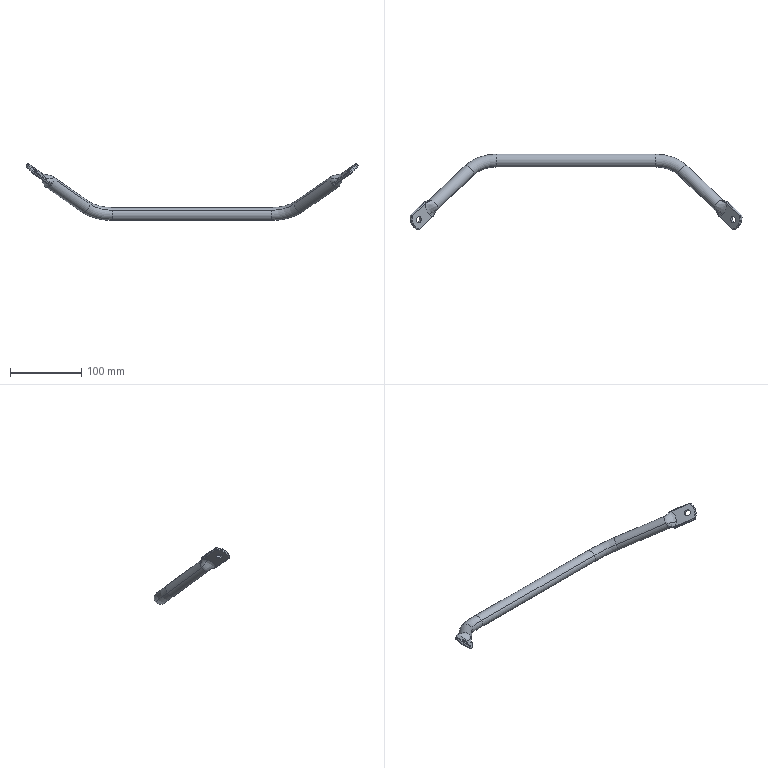Part | SolidWorks | 1 solid | 84 faces | box 465.151 x 106.147 x 79.693 mm | volume 56584 mm3 | cylinder 32 | spline 20 | torus 12 | sphere 12 | plane 8 | commonest cylinder face diameters 2 x12 14 x6 18 x6 9 x4 40 x4